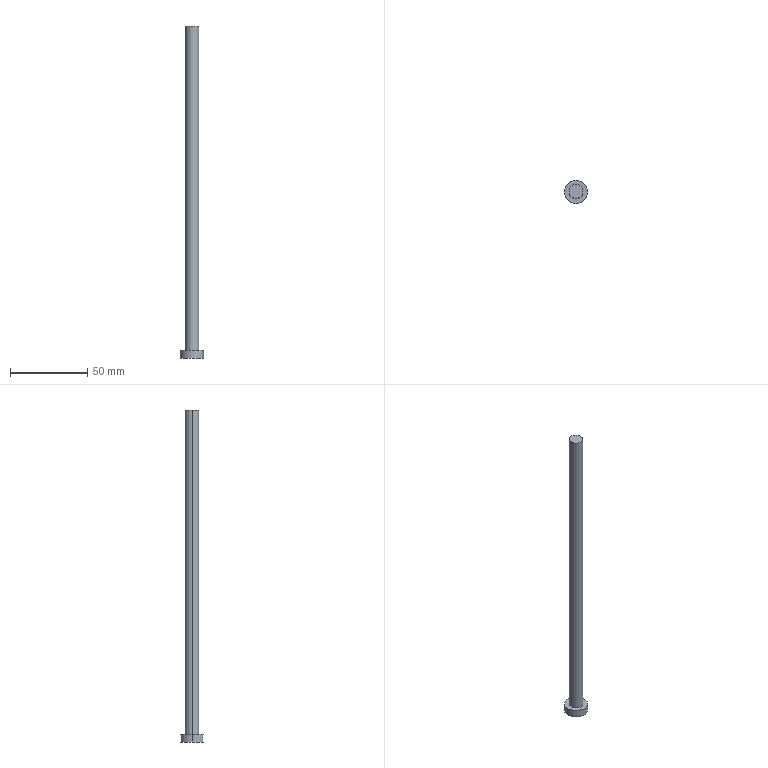Part | Creo | 1 solid | 7 faces | box 15 x 15 x 215 mm | volume 14243 mm3 | cylinder 4 | plane 3 | commonest cylinder face diameters 9 x2 15 x2
STEP:
#1=CARTESIAN_POINT('',(50.5,-235.,-230.5));
#2=VERTEX_POINT('',#1);
#3=CARTESIAN_POINT('',(59.5,-235.,-230.5));
#4=VERTEX_POINT('',#3);
#5=CARTESIAN_POINT('',(55.,-235.,-230.5));
#6=DIRECTION('',(0.,0.,-1.));
#7=DIRECTION('',(-1.,0.,0.));
#8=AXIS2_PLACEMENT_3D('',#5,#6,#7);
#9=CIRCLE('',#8,4.5);
#10=EDGE_CURVE('',#2,#4,#9,.T.);
#11=ORIENTED_EDGE('',*,*,#10,.T.);
#12=CARTESIAN_POINT('',(59.5,-235.,-20.5));
#13=VERTEX_POINT('',#12);
#14=CARTESIAN_POINT('',(59.5,-235.,-230.5));
#15=DIRECTION('',(0.,0.,1.));
#16=VECTOR('',#15,210.);
#17=LINE('',#14,#16);
#18=EDGE_CURVE('',#4,#13,#17,.T.);
#19=ORIENTED_EDGE('',*,*,#18,.T.);
#20=CARTESIAN_POINT('',(50.5,-235.,-20.5));
#21=VERTEX_POINT('',#20);
#22=CARTESIAN_POINT('',(55.,-235.,-20.5));
#23=DIRECTION('',(0.,0.,1.));
#24=DIRECTION('',(1.,0.,0.));
#25=AXIS2_PLACEMENT_3D('',#22,#23,#24);
#26=CIRCLE('',#25,4.5);
#27=EDGE_CURVE('',#13,#21,#26,.T.);
#28=ORIENTED_EDGE('',*,*,#27,.T.);
#29=CARTESIAN_POINT('',(50.5,-235.,-230.5));
#30=DIRECTION('',(0.,0.,1.));
#31=VECTOR('',#30,210.);
#32=LINE('',#29,#31);
#33=EDGE_CURVE('',#2,#21,#32,.T.);
#34=ORIENTED_EDGE('',*,*,#33,.F.);
#35=EDGE_LOOP('',(#11,#19,#28,#34));
#36=FACE_OUTER_BOUND('',#35,.F.);
#37=CARTESIAN_POINT('',(55.,-235.,-250.296));
#38=DIRECTION('',(0.,0.,1.));
#39=DIRECTION('',(1.,0.,0.));
#40=AXIS2_PLACEMENT_3D('',#37,#38,#39);
#41=CYLINDRICAL_SURFACE('',#40,4.5);
#42=ADVANCED_FACE('',(#36),#41,.T.);
#43=CARTESIAN_POINT('',(62.5,-235.,-230.5));
#44=VERTEX_POINT('',#43);
#45=CARTESIAN_POINT('',(47.5,-235.,-230.5));
#46=VERTEX_POINT('',#45);
#47=CARTESIAN_POINT('',(55.,-235.,-230.5));
#48=DIRECTION('',(0.,0.,1.));
#49=DIRECTION('',(1.,0.,0.));
#50=AXIS2_PLACEMENT_3D('',#47,#48,#49);
#51=CIRCLE('',#50,7.5);
#52=EDGE_CURVE('',#44,#46,#51,.T.);
#53=ORIENTED_EDGE('',*,*,#52,.F.);
#54=CARTESIAN_POINT('',(55.,-235.,-230.5));
#55=DIRECTION('',(0.,0.,1.));
#56=DIRECTION('',(-1.,0.,0.));
#57=AXIS2_PLACEMENT_3D('',#54,#55,#56);
#58=CIRCLE('',#57,7.5);
#59=EDGE_CURVE('',#46,#44,#58,.T.);
#60=ORIENTED_EDGE('',*,*,#59,.F.);
#61=EDGE_LOOP('',(#53,#60));
#62=FACE_OUTER_BOUND('',#61,.F.);
#63=CARTESIAN_POINT('',(55.,-235.,-230.5));
#64=DIRECTION('',(0.,0.,-1.));
#65=DIRECTION('',(1.,0.,0.));
#66=AXIS2_PLACEMENT_3D('',#63,#64,#65);
#67=CIRCLE('',#66,4.5);
#68=EDGE_CURVE('',#4,#2,#67,.T.);
#69=ORIENTED_EDGE('',*,*,#68,.F.);
#70=ORIENTED_EDGE('',*,*,#10,.F.);
#71=EDGE_LOOP('',(#69,#70));
#72=FACE_BOUND('',#71,.F.);
#73=CARTESIAN_POINT('',(55.,-235.,-230.5));
#74=DIRECTION('',(0.,0.,1.));
#75=DIRECTION('',(1.,0.,0.));
#76=AXIS2_PLACEMENT_3D('',#73,#74,#75);
#77=PLANE('',#76);
#78=ADVANCED_FACE('',(#62,#72),#77,.T.);
#79=CARTESIAN_POINT('',(47.5,-235.,-235.5));
#80=VERTEX_POINT('',#79);
#81=CARTESIAN_POINT('',(62.5,-235.,-235.5));
#82=VERTEX_POINT('',#81);
#83=CARTESIAN_POINT('',(55.,-235.,-235.5));
#84=DIRECTION('',(0.,0.,-1.));
#85=DIRECTION('',(-1.,0.,0.));
#86=AXIS2_PLACEMENT_3D('',#83,#84,#85);
#87=CIRCLE('',#86,7.5);
#88=EDGE_CURVE('',#80,#82,#87,.T.);
#89=ORIENTED_EDGE('',*,*,#88,.T.);
#90=CARTESIAN_POINT('',(62.5,-235.,-235.5));
#91=DIRECTION('',(0.,0.,1.));
#92=VECTOR('',#91,5.);
#93=LINE('',#90,#92);
#94=EDGE_CURVE('',#82,#44,#93,.T.);
#95=ORIENTED_EDGE('',*,*,#94,.T.);
#96=ORIENTED_EDGE('',*,*,#52,.T.);
#97=CARTESIAN_POINT('',(47.5,-235.,-235.5));
#98=DIRECTION('',(0.,0.,1.));
#99=VECTOR('',#98,5.);
#100=LINE('',#97,#99);
#101=EDGE_CURVE('',#80,#46,#100,.T.);
#102=ORIENTED_EDGE('',*,*,#101,.F.);
#103=EDGE_LOOP('',(#89,#95,#96,#102));
#104=FACE_OUTER_BOUND('',#103,.F.);
#105=CARTESIAN_POINT('',(55.,-235.,-241.77));
#106=DIRECTION('',(0.,0.,1.));
#107=DIRECTION('',(1.,0.,0.));
#108=AXIS2_PLACEMENT_3D('',#105,#106,#107);
#109=CYLINDRICAL_SURFACE('',#108,7.5);
#110=ADVANCED_FACE('',(#104),#109,.T.);
#111=CARTESIAN_POINT('',(55.,-235.,-235.5));
#112=DIRECTION('',(0.,0.,-1.));
#113=DIRECTION('',(1.,0.,0.));
#114=AXIS2_PLACEMENT_3D('',#111,#112,#113);
#115=CIRCLE('',#114,7.5);
#116=EDGE_CURVE('',#82,#80,#115,.T.);
#117=ORIENTED_EDGE('',*,*,#116,.F.);
#118=ORIENTED_EDGE('',*,*,#88,.F.);
#119=EDGE_LOOP('',(#117,#118));
#120=FACE_OUTER_BOUND('',#119,.F.);
#121=CARTESIAN_POINT('',(55.,-235.,-235.5));
#122=DIRECTION('',(0.,0.,1.));
#123=DIRECTION('',(1.,0.,0.));
#124=AXIS2_PLACEMENT_3D('',#121,#122,#123);
#125=PLANE('',#124);
#126=ADVANCED_FACE('',(#120),#125,.F.);
#127=ORIENTED_EDGE('',*,*,#116,.T.);
#128=ORIENTED_EDGE('',*,*,#101,.T.);
#129=ORIENTED_EDGE('',*,*,#59,.T.);
#130=ORIENTED_EDGE('',*,*,#94,.F.);
#131=EDGE_LOOP('',(#127,#128,#129,#130));
#132=FACE_OUTER_BOUND('',#131,.F.);
#133=CARTESIAN_POINT('',(55.,-235.,-241.77));
#134=DIRECTION('',(0.,0.,1.));
#135=DIRECTION('',(1.,0.,0.));
#136=AXIS2_PLACEMENT_3D('',#133,#134,#135);
#137=CYLINDRICAL_SURFACE('',#136,7.5);
#138=ADVANCED_FACE('',(#132),#137,.T.);
#139=ORIENTED_EDGE('',*,*,#68,.T.);
#140=ORIENTED_EDGE('',*,*,#33,.T.);
#141=CARTESIAN_POINT('',(55.,-235.,-20.5));
#142=DIRECTION('',(0.,0.,1.));
#143=DIRECTION('',(-1.,0.,0.));
#144=AXIS2_PLACEMENT_3D('',#141,#142,#143);
#145=CIRCLE('',#144,4.5);
#146=EDGE_CURVE('',#21,#13,#145,.T.);
#147=ORIENTED_EDGE('',*,*,#146,.T.);
#148=ORIENTED_EDGE('',*,*,#18,.F.);
#149=EDGE_LOOP('',(#139,#140,#147,#148));
#150=FACE_OUTER_BOUND('',#149,.F.);
#151=CARTESIAN_POINT('',(55.,-235.,-250.296));
#152=DIRECTION('',(0.,0.,1.));
#153=DIRECTION('',(1.,0.,0.));
#154=AXIS2_PLACEMENT_3D('',#151,#152,#153);
#155=CYLINDRICAL_SURFACE('',#154,4.5);
#156=ADVANCED_FACE('',(#150),#155,.T.);
#157=ORIENTED_EDGE('',*,*,#27,.F.);
#158=ORIENTED_EDGE('',*,*,#146,.F.);
#159=EDGE_LOOP('',(#157,#158));
#160=FACE_OUTER_BOUND('',#159,.F.);
#161=CARTESIAN_POINT('',(59.5,-235.,-20.5));
#162=DIRECTION('',(0.,0.,-1.));
#163=DIRECTION('',(-1.,0.,0.));
#164=AXIS2_PLACEMENT_3D('',#161,#162,#163);
#165=PLANE('',#164);
#166=ADVANCED_FACE('',(#160),#165,.F.);
#167=CLOSED_SHELL('',(#42,#78,#110,#126,#138,#156,#166));
#168=MANIFOLD_SOLID_BREP('',#167);
#169=(LENGTH_UNIT()NAMED_UNIT(*)SI_UNIT(.MILLI.,.METRE.));
#170=UNCERTAINTY_MEASURE_WITH_UNIT(LENGTH_MEASURE(0.0216),#169,'','');
#171=(NAMED_UNIT(*)PLANE_ANGLE_UNIT()SI_UNIT($,.RADIAN.));
#172=PLANE_ANGLE_MEASURE_WITH_UNIT(PLANE_ANGLE_MEASURE(0.01745),#171);
#173=(CONVERSION_BASED_UNIT('DEGREE',#172)NAMED_UNIT(*)PLANE_ANGLE_UNIT());
#174=(NAMED_UNIT(*)SI_UNIT($,.STERADIAN.)SOLID_ANGLE_UNIT());
#175=(GEOMETRIC_REPRESENTATION_CONTEXT(3)GLOBAL_UNCERTAINTY_ASSIGNED_CONTEXT((#170))GLOBAL_UNIT_ASSIGNED_CONTEXT((#169,#173,#174))REPRESENTATION_CONTEXT('',''));
#176=ADVANCED_BREP_SHAPE_REPRESENTATION('',(#168),#175);